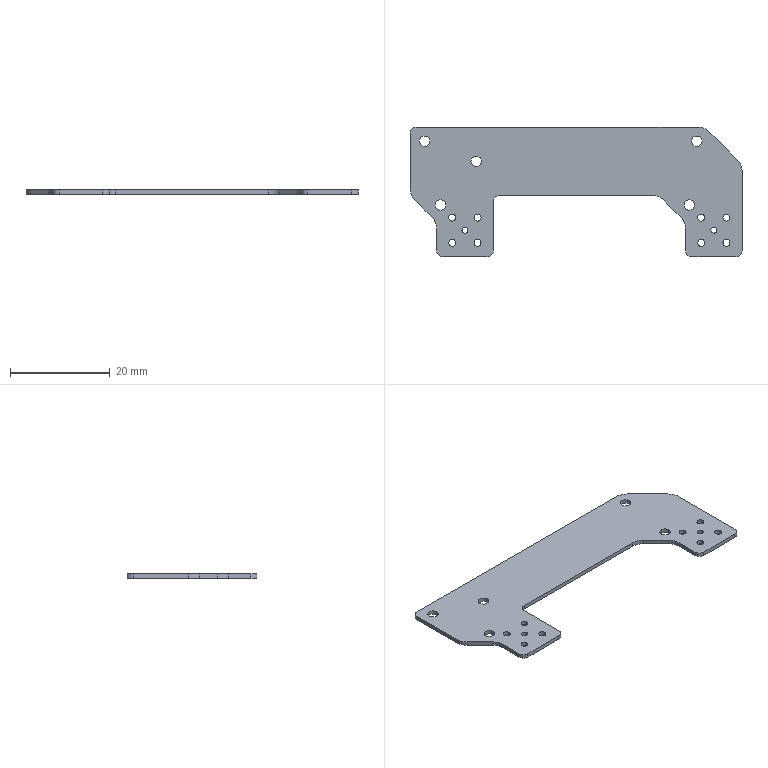Part | STEP file | 推动功放1分2PCB | 1 solid | 41 faces | box 66.71 x 26.09 x 0.832 mm | volume 967.615 mm3 | cylinder 27 | plane 14 | commonest cylinder face diameters 1.4 x8 2.54 x6 6.132 x6 2.1 x5 1.2 x2